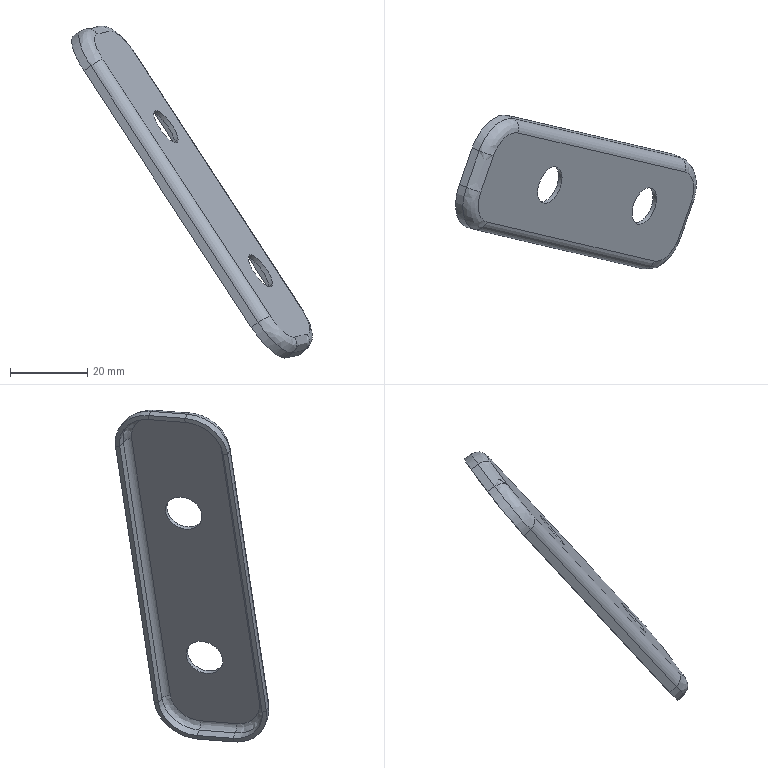Part | STEP file | FNA5401451 | 1 solid | 46 faces | box 62.39 x 39.872 x 86.052 mm | volume 4191 mm3 | spline 36 | cylinder 8 | plane 2 | commonest cylinder face diameters 10 x4 3.6 x2 6 x2